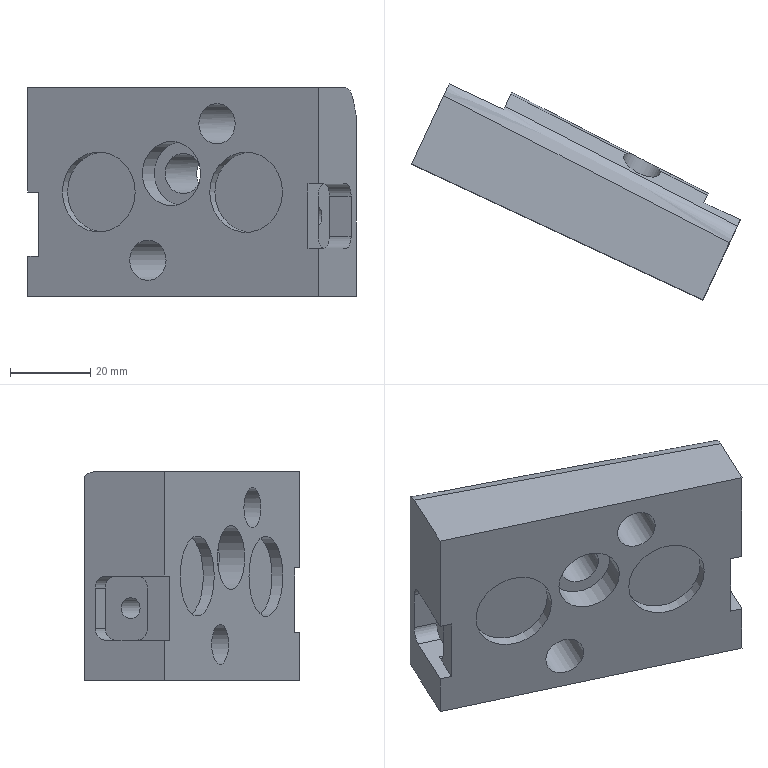Part | STEP file | gslz 2016.10.28-13_id1454_x_t | 1 solid | 47 faces | box 81.802 x 53.748 x 52 mm | volume 84086 mm3 | plane 24 | cylinder 16 | spline 5 | cone 2 | commonest cylinder face diameters 6 x8 5.2 x2 10 x2 20 x2 10.05 x1 16 x1